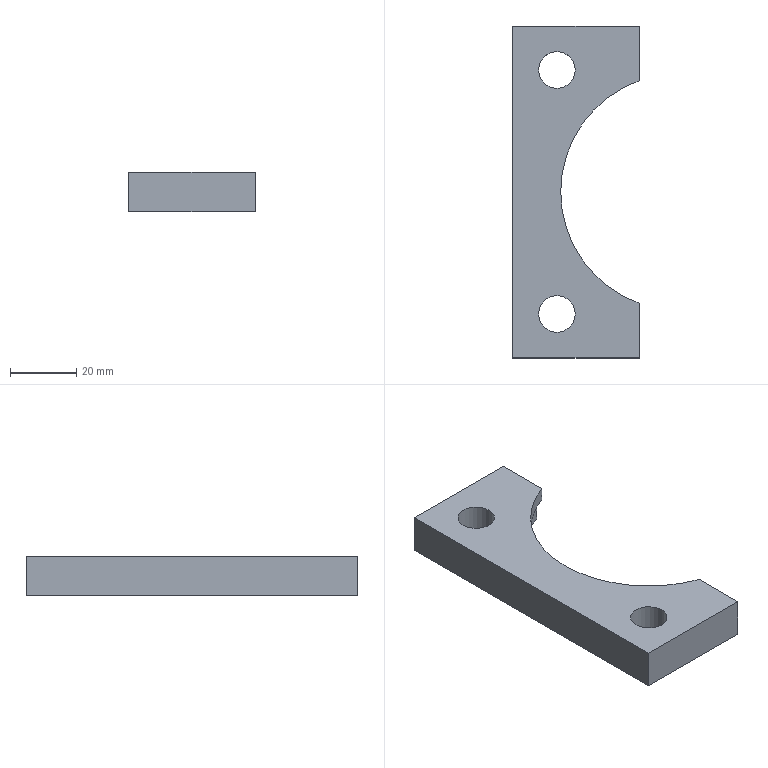Part | NX | features MAIN_BODY 2 | 1 solid | 12 faces | box 38 x 100 x 12 mm | volume 28037 mm3 | plane 8 | cylinder 4 | commonest cylinder face diameters 11 x2 71.2 x1 75.2 x1
STEP:
#1=CARTESIAN_POINT('',(-46.25,346.75,95.));
#2=VERTEX_POINT('',#1);
#3=CARTESIAN_POINT('',(-51.75,346.75,95.));
#4=DIRECTION('',(0.,0.,1.));
#5=DIRECTION('',(1.,0.,0.));
#6=AXIS2_PLACEMENT_3D('',#3,#4,#5);
#7=CIRCLE('',#6,5.5);
#8=EDGE_CURVE('',#2,#2,#7,.T.);
#9=ORIENTED_EDGE('',*,*,#8,.T.);
#10=EDGE_LOOP('',(#9));
#11=FACE_BOUND('',#10,.T.);
#12=CARTESIAN_POINT('',(-46.25,273.25,95.));
#13=VERTEX_POINT('',#12);
#14=CARTESIAN_POINT('',(-51.75,273.25,95.));
#15=DIRECTION('',(0.,0.,1.));
#16=DIRECTION('',(1.,0.,0.));
#17=AXIS2_PLACEMENT_3D('',#14,#15,#16);
#18=CIRCLE('',#17,5.5);
#19=EDGE_CURVE('',#13,#13,#18,.T.);
#20=ORIENTED_EDGE('',*,*,#19,.T.);
#21=EDGE_LOOP('',(#20));
#22=FACE_BOUND('',#21,.T.);
#23=CARTESIAN_POINT('',(-27.,360.,95.));
#24=VERTEX_POINT('',#23);
#25=CARTESIAN_POINT('',(-27.,345.634,95.));
#26=VERTEX_POINT('',#25);
#27=CARTESIAN_POINT('',(-27.,328.835,95.));
#28=DIRECTION('',(0.,-1.,0.));
#29=VECTOR('',#28,1000.);
#30=LINE('',#27,#29);
#31=EDGE_CURVE('',#24,#26,#30,.T.);
#32=ORIENTED_EDGE('',*,*,#31,.T.);
#33=CARTESIAN_POINT('',(-27.,274.366,95.));
#34=VERTEX_POINT('',#33);
#35=CARTESIAN_POINT('',(-15.,310.,95.));
#36=DIRECTION('',(0.,0.,1.));
#37=DIRECTION('',(1.,0.,0.));
#38=AXIS2_PLACEMENT_3D('',#35,#36,#37);
#39=CIRCLE('',#38,37.6);
#40=EDGE_CURVE('',#26,#34,#39,.T.);
#41=ORIENTED_EDGE('',*,*,#40,.T.);
#42=CARTESIAN_POINT('',(-27.,260.,95.));
#43=VERTEX_POINT('',#42);
#44=CARTESIAN_POINT('',(-27.,282.5,95.));
#45=DIRECTION('',(0.,1.,0.));
#46=VECTOR('',#45,1000.);
#47=LINE('',#44,#46);
#48=EDGE_CURVE('',#43,#34,#47,.T.);
#49=ORIENTED_EDGE('',*,*,#48,.F.);
#50=CARTESIAN_POINT('',(-65.,260.,95.));
#51=VERTEX_POINT('',#50);
#52=CARTESIAN_POINT('',(-17.5,260.,95.));
#53=DIRECTION('',(-1.,0.,0.));
#54=VECTOR('',#53,1000.);
#55=LINE('',#52,#54);
#56=EDGE_CURVE('',#43,#51,#55,.T.);
#57=ORIENTED_EDGE('',*,*,#56,.T.);
#58=CARTESIAN_POINT('',(-65.,360.,95.));
#59=VERTEX_POINT('',#58);
#60=CARTESIAN_POINT('',(-65.,282.5,95.));
#61=DIRECTION('',(0.,1.,0.));
#62=VECTOR('',#61,1000.);
#63=LINE('',#60,#62);
#64=EDGE_CURVE('',#51,#59,#63,.T.);
#65=ORIENTED_EDGE('',*,*,#64,.T.);
#66=CARTESIAN_POINT('',(-42.5,360.,95.));
#67=DIRECTION('',(1.,0.,0.));
#68=VECTOR('',#67,1000.);
#69=LINE('',#66,#68);
#70=EDGE_CURVE('',#59,#24,#69,.T.);
#71=ORIENTED_EDGE('',*,*,#70,.T.);
#72=EDGE_LOOP('',(#32,#41,#49,#57,#65,#71));
#73=FACE_BOUND('',#72,.T.);
#74=CARTESIAN_POINT('',(-15.,310.,95.));
#75=DIRECTION('',(0.,0.,-1.));
#76=DIRECTION('',(1.,0.,0.));
#77=AXIS2_PLACEMENT_3D('',#74,#75,#76);
#78=PLANE('',#77);
#79=ADVANCED_FACE('',(#11,#22,#73),#78,.T.);
#80=ORIENTED_EDGE('',*,*,#70,.F.);
#81=CARTESIAN_POINT('',(-65.,360.,107.));
#82=VERTEX_POINT('',#81);
#83=CARTESIAN_POINT('',(-65.,360.,101.5));
#84=DIRECTION('',(0.,0.,-1.));
#85=VECTOR('',#84,1000.);
#86=LINE('',#83,#85);
#87=EDGE_CURVE('',#82,#59,#86,.T.);
#88=ORIENTED_EDGE('',*,*,#87,.F.);
#89=CARTESIAN_POINT('',(-27.,360.,107.));
#90=VERTEX_POINT('',#89);
#91=CARTESIAN_POINT('',(-42.5,360.,107.));
#92=DIRECTION('',(-1.,0.,0.));
#93=VECTOR('',#92,1000.);
#94=LINE('',#91,#93);
#95=EDGE_CURVE('',#82,#90,#94,.F.);
#96=ORIENTED_EDGE('',*,*,#95,.T.);
#97=CARTESIAN_POINT('',(-27.,360.,101.5));
#98=DIRECTION('',(0.,0.,-1.));
#99=VECTOR('',#98,1000.);
#100=LINE('',#97,#99);
#101=EDGE_CURVE('',#90,#24,#100,.T.);
#102=ORIENTED_EDGE('',*,*,#101,.T.);
#103=EDGE_LOOP('',(#80,#88,#96,#102));
#104=FACE_BOUND('',#103,.T.);
#105=CARTESIAN_POINT('',(-42.5,360.,101.5));
#106=DIRECTION('',(0.,1.,0.));
#107=DIRECTION('',(-1.,0.,0.));
#108=AXIS2_PLACEMENT_3D('',#105,#106,#107);
#109=PLANE('',#108);
#110=ADVANCED_FACE('',(#104),#109,.T.);
#111=CARTESIAN_POINT('',(-27.,343.517,103.));
#112=VERTEX_POINT('',#111);
#113=CARTESIAN_POINT('',(-27.,343.517,107.));
#114=VERTEX_POINT('',#113);
#115=CARTESIAN_POINT('',(-27.,343.517,106.5));
#116=DIRECTION('',(0.,0.,1.));
#117=VECTOR('',#116,1000.);
#118=LINE('',#115,#117);
#119=EDGE_CURVE('',#112,#114,#118,.T.);
#120=ORIENTED_EDGE('',*,*,#119,.F.);
#121=CARTESIAN_POINT('',(-27.,345.634,103.));
#122=VERTEX_POINT('',#121);
#123=CARTESIAN_POINT('',(-27.,310.,103.));
#124=DIRECTION('',(0.,-1.,0.));
#125=VECTOR('',#124,1000.);
#126=LINE('',#123,#125);
#127=EDGE_CURVE('',#122,#112,#126,.T.);
#128=ORIENTED_EDGE('',*,*,#127,.F.);
#129=CARTESIAN_POINT('',(-27.,345.634,237.));
#130=DIRECTION('',(0.,0.,-1.));
#131=VECTOR('',#130,1000.);
#132=LINE('',#129,#131);
#133=EDGE_CURVE('',#122,#26,#132,.T.);
#134=ORIENTED_EDGE('',*,*,#133,.T.);
#135=ORIENTED_EDGE('',*,*,#31,.F.);
#136=ORIENTED_EDGE('',*,*,#101,.F.);
#137=CARTESIAN_POINT('',(-27.,328.835,107.));
#138=DIRECTION('',(0.,1.,0.));
#139=VECTOR('',#138,1000.);
#140=LINE('',#137,#139);
#141=EDGE_CURVE('',#90,#114,#140,.F.);
#142=ORIENTED_EDGE('',*,*,#141,.T.);
#143=EDGE_LOOP('',(#120,#128,#134,#135,#136,#142));
#144=FACE_BOUND('',#143,.T.);
#145=CARTESIAN_POINT('',(-27.,328.835,101.5));
#146=DIRECTION('',(1.,0.,0.));
#147=DIRECTION('',(0.,0.,1.));
#148=AXIS2_PLACEMENT_3D('',#145,#146,#147);
#149=PLANE('',#148);
#150=ADVANCED_FACE('',(#144),#149,.T.);
#151=CARTESIAN_POINT('',(-27.,274.366,103.));
#152=VERTEX_POINT('',#151);
#153=CARTESIAN_POINT('',(-27.,276.483,103.));
#154=VERTEX_POINT('',#153);
#155=CARTESIAN_POINT('',(-27.,310.,103.));
#156=DIRECTION('',(0.,1.,0.));
#157=VECTOR('',#156,1000.);
#158=LINE('',#155,#157);
#159=EDGE_CURVE('',#152,#154,#158,.T.);
#160=ORIENTED_EDGE('',*,*,#159,.T.);
#161=CARTESIAN_POINT('',(-27.,276.483,107.));
#162=VERTEX_POINT('',#161);
#163=CARTESIAN_POINT('',(-27.,276.483,106.5));
#164=DIRECTION('',(0.,0.,1.));
#165=VECTOR('',#164,1000.);
#166=LINE('',#163,#165);
#167=EDGE_CURVE('',#154,#162,#166,.T.);
#168=ORIENTED_EDGE('',*,*,#167,.T.);
#169=CARTESIAN_POINT('',(-27.,260.,107.));
#170=VERTEX_POINT('',#169);
#171=CARTESIAN_POINT('',(-27.,282.5,107.));
#172=DIRECTION('',(0.,-1.,0.));
#173=VECTOR('',#172,1000.);
#174=LINE('',#171,#173);
#175=EDGE_CURVE('',#170,#162,#174,.F.);
#176=ORIENTED_EDGE('',*,*,#175,.F.);
#177=CARTESIAN_POINT('',(-27.,260.,101.5));
#178=DIRECTION('',(0.,0.,-1.));
#179=VECTOR('',#178,1000.);
#180=LINE('',#177,#179);
#181=EDGE_CURVE('',#170,#43,#180,.T.);
#182=ORIENTED_EDGE('',*,*,#181,.T.);
#183=ORIENTED_EDGE('',*,*,#48,.T.);
#184=CARTESIAN_POINT('',(-27.,274.366,103.));
#185=DIRECTION('',(0.,0.,-1.));
#186=VECTOR('',#185,1000.);
#187=LINE('',#184,#186);
#188=EDGE_CURVE('',#152,#34,#187,.T.);
#189=ORIENTED_EDGE('',*,*,#188,.F.);
#190=EDGE_LOOP('',(#160,#168,#176,#182,#183,#189));
#191=FACE_BOUND('',#190,.T.);
#192=CARTESIAN_POINT('',(-27.,282.5,101.5));
#193=DIRECTION('',(-1.,0.,0.));
#194=DIRECTION('',(0.,-1.,0.));
#195=AXIS2_PLACEMENT_3D('',#192,#193,#194);
#196=PLANE('',#195);
#197=ADVANCED_FACE('',(#191),#196,.F.);
#198=ORIENTED_EDGE('',*,*,#56,.F.);
#199=ORIENTED_EDGE('',*,*,#181,.F.);
#200=CARTESIAN_POINT('',(-65.,260.,107.));
#201=VERTEX_POINT('',#200);
#202=CARTESIAN_POINT('',(-17.5,260.,107.));
#203=DIRECTION('',(1.,0.,0.));
#204=VECTOR('',#203,1000.);
#205=LINE('',#202,#204);
#206=EDGE_CURVE('',#170,#201,#205,.F.);
#207=ORIENTED_EDGE('',*,*,#206,.T.);
#208=CARTESIAN_POINT('',(-65.,260.,101.5));
#209=DIRECTION('',(0.,0.,-1.));
#210=VECTOR('',#209,1000.);
#211=LINE('',#208,#210);
#212=EDGE_CURVE('',#201,#51,#211,.T.);
#213=ORIENTED_EDGE('',*,*,#212,.T.);
#214=EDGE_LOOP('',(#198,#199,#207,#213));
#215=FACE_BOUND('',#214,.T.);
#216=CARTESIAN_POINT('',(-17.5,260.,101.5));
#217=DIRECTION('',(0.,-1.,0.));
#218=DIRECTION('',(1.,0.,0.));
#219=AXIS2_PLACEMENT_3D('',#216,#217,#218);
#220=PLANE('',#219);
#221=ADVANCED_FACE('',(#215),#220,.T.);
#222=ORIENTED_EDGE('',*,*,#64,.F.);
#223=ORIENTED_EDGE('',*,*,#212,.F.);
#224=CARTESIAN_POINT('',(-65.,282.5,107.));
#225=DIRECTION('',(0.,-1.,0.));
#226=VECTOR('',#225,1000.);
#227=LINE('',#224,#226);
#228=EDGE_CURVE('',#201,#82,#227,.F.);
#229=ORIENTED_EDGE('',*,*,#228,.T.);
#230=ORIENTED_EDGE('',*,*,#87,.T.);
#231=EDGE_LOOP('',(#222,#223,#229,#230));
#232=FACE_BOUND('',#231,.T.);
#233=CARTESIAN_POINT('',(-65.,282.5,101.5));
#234=DIRECTION('',(-1.,0.,0.));
#235=DIRECTION('',(0.,0.,-1.));
#236=AXIS2_PLACEMENT_3D('',#233,#234,#235);
#237=PLANE('',#236);
#238=ADVANCED_FACE('',(#232),#237,.T.);
#239=ORIENTED_EDGE('',*,*,#175,.T.);
#240=CARTESIAN_POINT('',(-15.,310.,107.));
#241=DIRECTION('',(0.,0.,-1.));
#242=DIRECTION('',(-1.,0.,0.));
#243=AXIS2_PLACEMENT_3D('',#240,#241,#242);
#244=CIRCLE('',#243,35.6);
#245=EDGE_CURVE('',#162,#114,#244,.T.);
#246=ORIENTED_EDGE('',*,*,#245,.T.);
#247=ORIENTED_EDGE('',*,*,#141,.F.);
#248=ORIENTED_EDGE('',*,*,#95,.F.);
#249=ORIENTED_EDGE('',*,*,#228,.F.);
#250=ORIENTED_EDGE('',*,*,#206,.F.);
#251=EDGE_LOOP('',(#239,#246,#247,#248,#249,#250));
#252=FACE_BOUND('',#251,.T.);
#253=CARTESIAN_POINT('',(-57.25,346.75,107.));
#254=VERTEX_POINT('',#253);
#255=CARTESIAN_POINT('',(-51.75,346.75,107.));
#256=DIRECTION('',(0.,0.,-1.));
#257=DIRECTION('',(-1.,0.,0.));
#258=AXIS2_PLACEMENT_3D('',#255,#256,#257);
#259=CIRCLE('',#258,5.5);
#260=EDGE_CURVE('',#254,#254,#259,.T.);
#261=ORIENTED_EDGE('',*,*,#260,.T.);
#262=EDGE_LOOP('',(#261));
#263=FACE_BOUND('',#262,.T.);
#264=CARTESIAN_POINT('',(-57.25,273.25,107.));
#265=VERTEX_POINT('',#264);
#266=CARTESIAN_POINT('',(-51.75,273.25,107.));
#267=DIRECTION('',(0.,0.,-1.));
#268=DIRECTION('',(-1.,0.,0.));
#269=AXIS2_PLACEMENT_3D('',#266,#267,#268);
#270=CIRCLE('',#269,5.5);
#271=EDGE_CURVE('',#265,#265,#270,.T.);
#272=ORIENTED_EDGE('',*,*,#271,.T.);
#273=EDGE_LOOP('',(#272));
#274=FACE_BOUND('',#273,.T.);
#275=CARTESIAN_POINT('',(-15.,310.,107.));
#276=DIRECTION('',(0.,0.,1.));
#277=DIRECTION('',(-1.,0.,0.));
#278=AXIS2_PLACEMENT_3D('',#275,#276,#277);
#279=PLANE('',#278);
#280=ADVANCED_FACE('',(#252,#263,#274),#279,.T.);
#281=ORIENTED_EDGE('',*,*,#127,.T.);
#282=CARTESIAN_POINT('',(-15.,310.,103.));
#283=DIRECTION('',(0.,0.,-1.));
#284=DIRECTION('',(-1.,0.,0.));
#285=AXIS2_PLACEMENT_3D('',#282,#283,#284);
#286=CIRCLE('',#285,35.6);
#287=EDGE_CURVE('',#112,#154,#286,.F.);
#288=ORIENTED_EDGE('',*,*,#287,.T.);
#289=ORIENTED_EDGE('',*,*,#159,.F.);
#290=CARTESIAN_POINT('',(-15.,310.,103.));
#291=DIRECTION('',(0.,0.,-1.));
#292=DIRECTION('',(-1.,0.,0.));
#293=AXIS2_PLACEMENT_3D('',#290,#291,#292);
#294=CIRCLE('',#293,37.6);
#295=EDGE_CURVE('',#122,#152,#294,.F.);
#296=ORIENTED_EDGE('',*,*,#295,.F.);
#297=EDGE_LOOP('',(#281,#288,#289,#296));
#298=FACE_BOUND('',#297,.T.);
#299=CARTESIAN_POINT('',(-15.,310.,103.));
#300=DIRECTION('',(0.,0.,1.));
#301=DIRECTION('',(-1.,0.,0.));
#302=AXIS2_PLACEMENT_3D('',#299,#300,#301);
#303=PLANE('',#302);
#304=ADVANCED_FACE('',(#298),#303,.F.);
#305=ORIENTED_EDGE('',*,*,#119,.T.);
#306=ORIENTED_EDGE('',*,*,#245,.F.);
#307=ORIENTED_EDGE('',*,*,#167,.F.);
#308=ORIENTED_EDGE('',*,*,#287,.F.);
#309=EDGE_LOOP('',(#305,#306,#307,#308));
#310=FACE_BOUND('',#309,.T.);
#311=CARTESIAN_POINT('',(-15.,310.,106.5));
#312=DIRECTION('',(0.,0.,1.));
#313=DIRECTION('',(-1.,0.,0.));
#314=AXIS2_PLACEMENT_3D('',#311,#312,#313);
#315=CYLINDRICAL_SURFACE('',#314,35.6);
#316=ADVANCED_FACE('',(#310),#315,.F.);
#317=ORIENTED_EDGE('',*,*,#295,.T.);
#318=ORIENTED_EDGE('',*,*,#188,.T.);
#319=ORIENTED_EDGE('',*,*,#40,.F.);
#320=ORIENTED_EDGE('',*,*,#133,.F.);
#321=EDGE_LOOP('',(#317,#318,#319,#320));
#322=FACE_BOUND('',#321,.T.);
#323=CARTESIAN_POINT('',(-15.,310.,237.));
#324=DIRECTION('',(0.,0.,-1.));
#325=DIRECTION('',(1.,0.,0.));
#326=AXIS2_PLACEMENT_3D('',#323,#324,#325);
#327=CYLINDRICAL_SURFACE('',#326,37.6);
#328=ADVANCED_FACE('',(#322),#327,.F.);
#329=ORIENTED_EDGE('',*,*,#271,.F.);
#330=EDGE_LOOP('',(#329));
#331=FACE_BOUND('',#330,.T.);
#332=ORIENTED_EDGE('',*,*,#19,.F.);
#333=EDGE_LOOP('',(#332));
#334=FACE_BOUND('',#333,.T.);
#335=CARTESIAN_POINT('',(-51.75,273.25,107.));
#336=DIRECTION('',(0.,0.,-1.));
#337=DIRECTION('',(1.,0.,0.));
#338=AXIS2_PLACEMENT_3D('',#335,#336,#337);
#339=CYLINDRICAL_SURFACE('',#338,5.5);
#340=ADVANCED_FACE('',(#331,#334),#339,.F.);
#341=ORIENTED_EDGE('',*,*,#260,.F.);
#342=EDGE_LOOP('',(#341));
#343=FACE_BOUND('',#342,.T.);
#344=ORIENTED_EDGE('',*,*,#8,.F.);
#345=EDGE_LOOP('',(#344));
#346=FACE_BOUND('',#345,.T.);
#347=CARTESIAN_POINT('',(-51.75,346.75,107.));
#348=DIRECTION('',(0.,0.,-1.));
#349=DIRECTION('',(1.,0.,0.));
#350=AXIS2_PLACEMENT_3D('',#347,#348,#349);
#351=CYLINDRICAL_SURFACE('',#350,5.5);
#352=ADVANCED_FACE('',(#343,#346),#351,.F.);
#353=CLOSED_SHELL('',(#79,#110,#150,#197,#221,#238,#280,#304,#316,#328,#340,#352));
#354=MANIFOLD_SOLID_BREP('',#353);
#355=(LENGTH_UNIT()NAMED_UNIT(*)SI_UNIT(.MILLI.,.METRE.));
#356=UNCERTAINTY_MEASURE_WITH_UNIT(LENGTH_MEASURE(0.00001),#355,'','');
#357=(NAMED_UNIT(*)PLANE_ANGLE_UNIT()SI_UNIT($,.RADIAN.));
#358=(NAMED_UNIT(*)SI_UNIT($,.STERADIAN.)SOLID_ANGLE_UNIT());
#359=(GEOMETRIC_REPRESENTATION_CONTEXT(3)GLOBAL_UNCERTAINTY_ASSIGNED_CONTEXT((#356))GLOBAL_UNIT_ASSIGNED_CONTEXT((#355,#357,#358))REPRESENTATION_CONTEXT('',''));
#360=ADVANCED_BREP_SHAPE_REPRESENTATION('',(#354),#359);